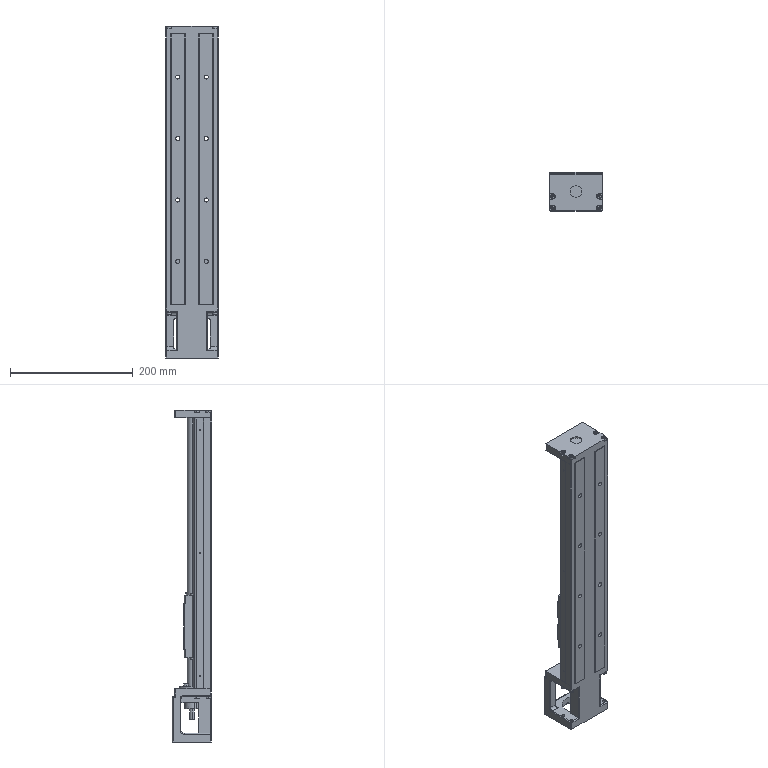Part | NX | features BREP 2 | 2 solids | 586 faces | box 86 x 64 x 540 mm | volume 1109706 mm3 | plane 309 | cylinder 226 | cone 34 | sphere 9 | torus 8 | commonest cylinder face diameters 7.5 x32 3 x31 6 x22 3.3 x18 2.15 x16 4.5 x16